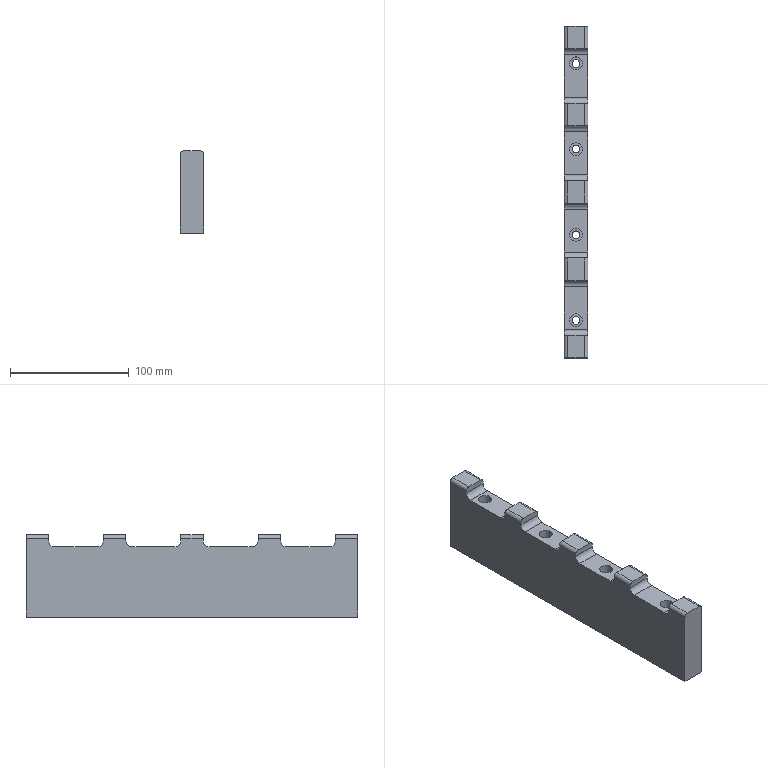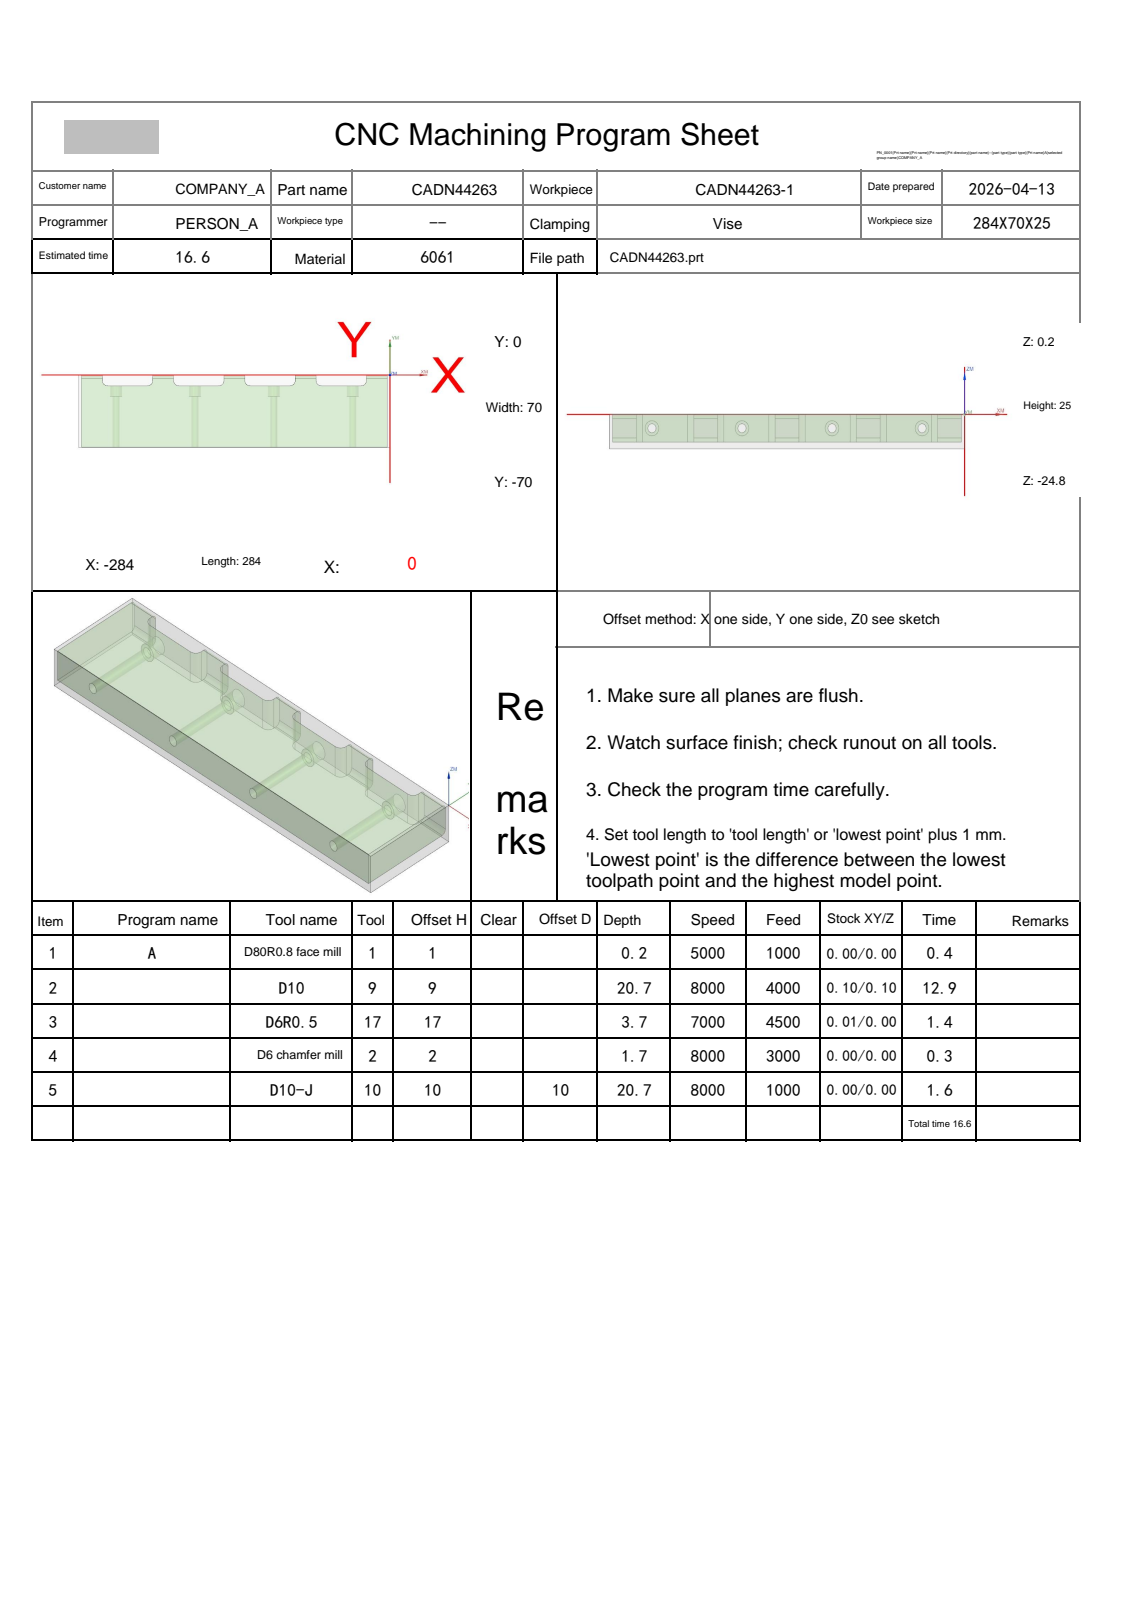NC program | NX | posted by the shop | part box 20 x 279 x 69 mm
Lines 32 to 993 of 9859:
N2 T09 M06
(D10  D=10. R=0. H=09 ce=0.10 di=0.10)
G00 G90 G54 X-229.134 Y12. M03 S8000
G43 H09 Z10.2
M08
Z.614
G01 Z-.586 F4000.
G02 X-228.084 Y8.312 I-5.95 J-3.688
X-228.918 Y5. I-7. J0.0
G03 X-229.323 Y4.183 I12.45 J-6.687
G02 X-230.23 Y3.6 I-.909 J.417
G01 X-248.795
G02 X-249.701 Y4.18 I.002 J1.
G03 X-250.111 Y5. I-12.905 J-5.942
G02 X-250.955 Y8.331 I6.156 J3.331
X-249.917 Y12. I7. J0.0
G01 Z.614
G00 Z3.
G01 X-164.121 F6000.
G00 Z.614
G01 Z-.586 F4000.
G02 X-163.073 Y8.315 I-5.952 J-3.685
X-163.908 Y5. I-7. J0.0
G03 X-164.314 Y4.183 I12.457 J-6.699
G02 X-165.221 Y3.6 I-.909 J.417
G01 X-183.777
G02 X-184.684 Y4.182 I.002 J1.
G03 X-185.091 Y5. I-12.87 J-5.892
G02 X-185.927 Y8.318 I6.164 J3.318
X-184.881 Y12. I7. J0.0
G01 Z.614
G00 Z3.
G01 X-99.102 F6000.
G00 Z.614
G01 Z-.586 F4000.
G02 X-98.06 Y8.324 I-5.957 J-3.676
X-98.9 Y5. I-7. J0.0
G03 X-99.308 Y4.181 I12.478 J-6.734
G02 X-100.214 Y3.6 I-.908 J.419
G01 X-118.771
G02 X-119.679 Y4.185 I.002 J1.
G03 X-120.081 Y5. I-12.821 J-5.821
G02 X-120.907 Y8.299 I6.174 J3.299
X-119.849 Y12. I7. J0.0
G01 Z.614
G00 Z3.
G01 X-34.092 F6000.
G00 Z.614
G01 Z-.586 F4000.
G02 X-33.051 Y8.328 I-5.96 J-3.672
X-33.893 Y5. I-7. J0.0
G03 X-34.303 Y4.181 I12.488 J-6.75
G02 X-35.209 Y3.6 I-.908 J.419
G01 X-53.77
G02 X-54.671 Y4.17 I.002 J1.
G03 X-55.573 Y4.739 I-.903 J-.431
X-55.932 Y4.673 I0.0 J-1.
G01 X-62.489 Y2.148
G03 X-63.13 Y1.214 I.359 J-.933
X-63.011 Y.741 I1. J0.0
G02 X-62.4 Y-1.687 I-4.521 J-2.429
G01 Y-1.72
Y-2.023
G03 X-62.225 Y-2.242 I.224 J0.0
G02 X-61.631 Y-2.785 I-.177 J-.79
G03 X-59.25 Y-4.523 I2.381 J.762
X-57.559 Y-3.865 I0.0 J2.5
G01 X-53.852 Y-.461
G03 X-53.043 Y1.381 I-1.691 J1.841
X-55.543 Y3.881 I-2.5 J0.0
X-57.234 Y3.222 I0.0 J-2.5
G01 X-60.941 Y-.182
G03 X-61.684 Y-1.452 I1.691 J-1.841
G02 X-61.993 Y-1.756 I-.394 J.093
G01 X-62.223 Y-1.805
G03 X-62.4 Y-2.023 I.047 J-.219
G01 Y-3.419
G02 X-62.379 Y-4.409 I-23.84 J-.991
X-62.4 Y-5.4 I-23.861 J0.0
G01 X-26.6
Y-2.028
G03 X-26.774 Y-1.81 I-.223 J0.0
G02 X-27.365 Y-1.269 I.177 J.787
G03 X-28.052 Y-.191 I-2.382 J-.759
G01 X-31.744 Y3.217
G03 X-33.439 Y3.88 I-1.696 J-1.837
X-35.939 Y1.38 I0.0 J-2.5
X-35.135 Y-.457 I2.5 J0.0
G01 X-31.443 Y-3.865
G03 X-29.747 Y-4.528 I1.696 J1.837
X-27.313 Y-2.597 I0.0 J2.5
G02 X-27.005 Y-2.294 I.393 J-.092
G01 X-26.776 Y-2.246
G03 X-26.6 Y-2.028 I-.046 J.218
G01 Y-1.844
X-26.601 Y-1.75
G02 X-21.5 Y3.445 I5.195 J0.0
G01 X-2.5
G02 X2.6 Y-1.713 I-.057 J-5.157
G01 Y-1.72
Y-69.443
Y-69.498
G02 X2.505 Y-70.479 I-5.101 J0.0
X-2.5 Y-74.6 I-5.005 J.979
G01 X-281.5
G02 X-286.505 Y-70.479 I0.0 J5.1
X-286.6 Y-69.498 I5.006 J.981
G01 Y-69.443
Y-1.72
Y-1.717
G02 X-281.5 Y3.445 I5.162 J0.0
G01 X-262.5
G02 X-257.399 Y-1.762 I-.107 J-5.207
G01 X-257.4 Y-1.869
Y-2.029
G03 X-257.226 Y-2.246 I.223 J0.0
G02 X-256.635 Y-2.787 I-.177 J-.786
G03 X-254.253 Y-4.529 I2.382 J.758
X-252.557 Y-3.865 I0.0 J2.5
G01 X-248.868 Y-.457
G03 X-248.064 Y1.379 I-1.696 J1.836
X-250.564 Y3.879 I-2.5 J0.0
X-252.261 Y3.216 I0.0 J-2.5
G01 X-255.95 Y-.192
G03 X-256.688 Y-1.46 I1.696 J-1.836
G02 X-256.995 Y-1.762 I-.392 J.092
G01 X-257.224 Y-1.811
G03 X-257.4 Y-2.029 I.046 J-.218
G01 Y-3.403
G02 X-257.378 Y-4.402 I-22.182 J-.998
X-257.4 Y-5.4 I-22.205 J0.0
G01 X-221.6
Y-2.023
G03 X-221.775 Y-1.805 I-.224 J0.0
G02 X-222.369 Y-1.262 I.177 J.79
G03 X-223.059 Y-.182 I-2.381 J-.762
G01 X-226.766 Y3.222
G03 X-228.457 Y3.881 I-1.691 J-1.841
X-230.957 Y1.381 I0.0 J-2.5
X-230.148 Y-.461 I2.5 J0.0
G01 X-226.441 Y-3.865
G03 X-224.75 Y-4.523 I1.691 J1.841
X-222.316 Y-2.594 I0.0 J2.5
G02 X-222.007 Y-2.291 I.394 J-.093
G01 X-221.777 Y-2.242
G03 X-221.6 Y-2.023 I-.047 J.219
G01 Y-1.72
Y-1.687
G02 X-216.5 Y3.445 I5.132 J0.0
G01 X-197.5
G02 X-192.4 Y-1.709 I-.054 J-5.154
G01 Y-1.763
Y-2.025
G03 X-192.225 Y-2.243 I.223 J0.0
G02 X-191.632 Y-2.785 I-.177 J-.789
G03 X-189.251 Y-4.525 I2.381 J.761
X-187.558 Y-3.865 I0.0 J2.5
G01 X-183.857 Y-.459
G03 X-183.049 Y1.38 I-1.693 J1.84
X-185.549 Y3.88 I-2.5 J0.0
X-187.242 Y3.22 I0.0 J-2.5
G01 X-190.943 Y-.185
G03 X-191.685 Y-1.455 I1.693 J-1.84
G02 X-191.994 Y-1.758 I-.394 J.092
G01 X-192.223 Y-1.807
G03 X-192.4 Y-2.025 I.047 J-.218
G01 Y-3.41
G02 X-192.382 Y-4.405 I-27.479 J-.995
X-192.4 Y-5.4 I-27.497 J0.0
G01 X-156.6
Y-5.388
G02 X-156.627 Y-4.37 I19.024 J1.018
X-156.6 Y-3.351 I19.052 J0.0
G01 Y-2.026
G03 X-156.773 Y-1.81 I-.222 J0.0
G02 X-157.362 Y-1.269 I.176 J.783
G03 X-158.051 Y-.187 I-2.383 J-.757
G01 X-161.752 Y3.222
G03 X-163.446 Y3.883 I-1.694 J-1.839
X-165.946 Y1.383 I0.0 J-2.5
X-165.14 Y-.456 I2.5 J0.0
G01 X-161.439 Y-3.865
G03 X-159.745 Y-4.526 I1.694 J1.839
X-157.31 Y-2.593 I0.0 J2.5
G02 X-157.003 Y-2.292 I.391 J-.091
G01 X-156.775 Y-2.243
G03 X-156.6 Y-2.026 I-.046 J.217
G01 Y-1.779
G02 X-156.454 Y-.505 I5.64 J0.0
X-151.5 Y3.445 I5.003 J-1.194
G01 X-132.5
G02 X-127.448 Y-1.094 I0.0 J-5.08
X-127.4 Y-2.002 I-8.464 J-.907
G01 Y-2.02
G03 X-127.23 Y-2.232 I.218 J0.0
G02 X-126.653 Y-2.766 I-.175 J-.769
G03 X-124.267 Y-4.52 I2.386 J.746
X-122.58 Y-3.865 I0.0 J2.5
G01 X-118.86 Y-.463
G03 X-118.047 Y1.382 I-1.687 J1.845
X-120.547 Y3.882 I-2.5 J0.0
X-122.234 Y3.227 I0.0 J-2.5
G01 X-125.954 Y-.175
G03 X-126.704 Y-1.462 I1.687 J-1.845
G02 X-127.005 Y-1.759 I-.384 J.088
G01 X-127.228 Y-1.807
G03 X-127.4 Y-2.02 I.046 J-.213
G01 Y-3.351
G02 X-127.372 Y-4.376 I-19.025 J-1.024
X-127.4 Y-5.4 I-19.052 J0.0
G01 X-91.6
Y-2.027
G03 X-91.774 Y-1.809 I-.223 J0.0
G02 X-92.366 Y-1.267 I.177 J.788
G03 X-93.054 Y-.188 I-2.382 J-.76
G01 X-96.749 Y3.218
G03 X-98.444 Y3.88 I-1.694 J-1.838
X-100.944 Y1.38 I0.0 J-2.5
X-100.138 Y-.458 I2.5 J0.0
G01 X-96.443 Y-3.865
G03 X-94.748 Y-4.527 I1.694 J1.838
X-92.314 Y-2.596 I0.0 J2.5
G02 X-92.005 Y-2.294 I.393 J-.092
G01 X-91.776 Y-2.245
G03 X-91.6 Y-2.027 I-.047 J.218
G01 Y-1.812
X-91.601 Y-1.734
G02 X-86.5 Y3.445 I5.179 J0.0
G01 X-67.5
G02 X-62.4 Y-1.687 I-.032 J-5.132
G01 Y-1.72
Y-3.419
G02 X-62.381 Y-4.157 I-23.84 J-.986
X-62.38 Y-4.405 I-23.859 J-.248
X-62.381 Y-4.657 I-23.861 J0.0
G03 X-55.381 Y2.343 I0.0 J7.
G01 Y12.
Z.614
G00 Z3.
G01 X-229.72 F6000.
G00 Z.029
G01 Z-1.171 F4000.
G02 X-228.495 Y8.044 I-5.775 J-3.956
X-229.191 Y5. I-7. J0.0
G03 X-229.54 Y4.218 I12.752 J-6.157
G02 X-230.462 Y3.6 I-.924 J.382
G01 X-248.523
G02 X-249.445 Y4.22 I.003 J1.
G03 X-249.791 Y5. I-13.068 J-5.329
G02 X-250.481 Y8.03 I6.31 J3.03
X-249.246 Y12. I7. J0.0
G01 Z.029
G00 Z2.414
G01 X-164.725 F6000.
G00 Z.029
G01 Z-1.171 F4000.
G02 X-163.499 Y8.042 I-5.774 J-3.958
X-164.194 Y5. I-7. J0.0
G03 X-164.543 Y4.218 I12.748 J-6.151
G02 X-165.464 Y3.6 I-.924 J.382
G01 X-183.523
G02 X-184.445 Y4.22 I.003 J1.
G03 X-184.791 Y5. I-13.068 J-5.329
G02 X-185.481 Y8.03 I6.31 J3.03
X-184.246 Y12. I7. J0.0
G01 Z.029
G00 Z2.414
G01 X-99.754 F6000.
G00 Z.029
G01 Z-1.171 F4000.
G02 X-98.519 Y8.03 I-5.765 J-3.97
X-99.209 Y5. I-7. J0.0
G03 X-99.555 Y4.22 I12.722 J-6.109
G02 X-100.477 Y3.6 I-.925 J.38
G01 X-118.523
G02 X-119.445 Y4.22 I.003 J1.
G03 X-119.791 Y5. I-13.068 J-5.329
G02 X-120.481 Y8.03 I6.31 J3.03
X-119.246 Y12. I7. J0.0
G01 Z.029
G00 Z2.414
G01 X-34.754 F6000.
G00 Z.029
G01 Z-1.171 F4000.
G02 X-33.519 Y8.03 I-5.765 J-3.97
X-34.209 Y5. I-7. J0.0
G03 X-34.555 Y4.22 I12.722 J-6.109
G02 X-35.477 Y3.6 I-.925 J.38
G01 X-53.538
G02 X-54.444 Y4.181 I.003 J1.
G03 X-55.352 Y4.762 I-.908 J-.419
X-55.67 Y4.71 I0.0 J-1.
G01 X-62.332 Y2.469
G03 X-63.013 Y1.522 I.319 J-.948
X-62.913 Y1.087 I1. J0.0
G02 X-62.4 Y-1.121 I-4.648 J-2.244
G01 Y-1.989
G03 X-62.218 Y-2.215 I.232 J0.0
G02 X-61.601 Y-2.772 I-.18 J-.82
G03 X-59.227 Y-4.489 I2.374 J.783
X-57.572 Y-3.863 I0.0 J2.5
G01 X-53.717 Y-.458
G03 X-52.873 Y1.416 I-1.655 J1.874
X-55.373 Y3.916 I-2.5 J0.0
X-57.028 Y3.29 I0.0 J-2.5
G01 X-60.882 Y-.115
G03 X-61.656 Y-1.4 I1.655 J-1.874
G02 X-61.977 Y-1.711 I-.408 J.099
G01 X-62.216 Y-1.762
G03 X-62.4 Y-1.989 I.048 J-.227
G01 Y-3.419
G02 X-62.379 Y-4.409 I-23.84 J-.991
X-62.4 Y-5.4 I-23.861 J0.0
G01 X-26.6
Y-1.985
G03 X-26.782 Y-1.759 I-.232 J0.0
G02 X-27.399 Y-1.202 I.18 J.82
G03 X-28.122 Y-.108 I-2.374 J-.783
G01 X-31.989 Y3.294
G03 X-33.64 Y3.917 I-1.651 J-1.877
X-36.14 Y1.417 I0.0 J-2.5
X-35.292 Y-.46 I2.5 J0.0
G01 X-31.425 Y-3.862
G03 X-29.773 Y-4.485 I1.651 J1.877
X-27.344 Y-2.574 I0.0 J2.5
G02 X-27.023 Y-2.263 I.408 J-.099
G01 X-26.784 Y-2.212
G03 X-26.6 Y-1.985 I-.048 J.227
G01 Y-1.121
Y-1.109
G02 X-21.5 Y4.003 I5.112 J0.0
G01 X-2.5
G02 X2.6 Y-1.109 I-.012 J-5.112
G01 Y-1.121
Y-69.443
Y-69.498
G02 X2.505 Y-70.479 I-5.101 J0.0
X-2.5 Y-74.6 I-5.005 J.979
G01 X-281.5
G02 X-286.505 Y-70.479 I0.0 J5.1
X-286.6 Y-69.498 I5.006 J.981
G01 Y-69.443
Y-1.121
Y-1.109
G02 X-281.5 Y4.003 I5.112 J0.0
G01 X-262.5
G02 X-257.4 Y-1.109 I-.012 J-5.112
G01 Y-1.121
Y-1.655
X-257.398 Y-1.749
G03 X-257.18 Y-2.092 I.386 J.005
G01 X-256.944 Y-2.205
G02 X-256.66 Y-2.559 I-.23 J-.475
G03 X-254.227 Y-4.485 I2.433 J.574
X-252.575 Y-3.862 I0.0 J2.5
G01 X-248.708 Y-.46
G03 X-247.86 Y1.417 I-1.651 J1.877
X-250.36 Y3.917 I-2.5 J0.0
X-252.011 Y3.294 I0.0 J-2.5
G01 X-255.878 Y-.108
G03 X-256.656 Y-1.396 I1.651 J-1.877
G02 X-256.977 Y-1.708 I-.408 J.099
G01 X-257.216 Y-1.759
G03 X-257.4 Y-1.985 I.048 J-.227
G01 Y-3.403
G02 X-257.378 Y-4.402 I-22.182 J-.998
X-257.4 Y-5.4 I-22.205 J0.0
G01 X-221.6
Y-1.989
G03 X-221.782 Y-1.763 I-.232 J0.0
G02 X-222.399 Y-1.206 I.18 J.82
G03 X-223.118 Y-.115 I-2.374 J-.783
G01 X-226.972 Y3.29
G03 X-228.627 Y3.916 I-1.655 J-1.874
X-231.127 Y1.416 I0.0 J-2.5
X-230.283 Y-.458 I2.5 J0.0
G01 X-226.428 Y-3.863
G03 X-224.773 Y-4.489 I1.655 J1.874
X-222.344 Y-2.578 I0.0 J2.5
G02 X-222.023 Y-2.267 I.408 J-.099
G01 X-221.784 Y-2.216
G03 X-221.6 Y-1.989 I-.048 J.227
G01 Y-1.121
G02 X-216.5 Y4.003 I5.161 J-.036
G01 X-197.5
G02 X-192.4 Y-1.109 I-.012 J-5.112
G01 Y-1.121
Y-1.985
G03 X-192.218 Y-2.212 I.232 J0.0
G02 X-191.601 Y-2.768 I-.18 J-.82
G03 X-189.227 Y-4.485 I2.374 J.783
X-187.575 Y-3.862 I0.0 J2.5
G01 X-183.708 Y-.46
G03 X-182.86 Y1.417 I-1.651 J1.877
X-185.36 Y3.917 I-2.5 J0.0
X-187.011 Y3.294 I0.0 J-2.5
G01 X-190.878 Y-.108
G03 X-191.656 Y-1.396 I1.651 J-1.877
G02 X-191.977 Y-1.708 I-.408 J.099
G01 X-192.216 Y-1.759
G03 X-192.4 Y-1.985 I.048 J-.227
G01 Y-3.41
G02 X-192.382 Y-4.405 I-27.479 J-.995
X-192.4 Y-5.4 I-27.497 J0.0
G01 X-156.6
Y-5.388
G02 X-156.627 Y-4.37 I19.024 J1.018
X-156.6 Y-3.351 I19.052 J0.0
G01 Y-1.989
G03 X-156.782 Y-1.762 I-.232 J0.0
G02 X-157.4 Y-1.205 I.18 J.82
G03 X-158.119 Y-.114 I-2.374 J-.783
G01 X-161.975 Y3.29
G03 X-163.629 Y3.916 I-1.655 J-1.874
X-166.129 Y1.416 I0.0 J-2.5
X-165.284 Y-.458 I2.5 J0.0
G01 X-161.428 Y-3.863
G03 X-159.774 Y-4.489 I1.655 J1.874
X-157.344 Y-2.578 I0.0 J2.5
G02 X-157.024 Y-2.266 I.408 J-.099
G01 X-156.784 Y-2.215
G03 X-156.6 Y-1.989 I-.048 J.227
G01 Y-1.62
Y-1.121
G02 X-151.5 Y4.003 I5.155 J-.03
G01 X-132.5
G02 X-127.4 Y-1.109 I-.012 J-5.112
G01 Y-1.121
Y-1.985
G03 X-127.218 Y-2.212 I.232 J0.0
G02 X-126.601 Y-2.768 I-.18 J-.82
G03 X-124.227 Y-4.485 I2.374 J.783
X-122.575 Y-3.862 I0.0 J2.5
G01 X-118.708 Y-.46
G03 X-117.86 Y1.417 I-1.651 J1.877
X-120.36 Y3.917 I-2.5 J0.0
X-122.011 Y3.294 I0.0 J-2.5
G01 X-125.878 Y-.108
G03 X-126.656 Y-1.396 I1.651 J-1.877
G02 X-126.977 Y-1.708 I-.408 J.099
G01 X-127.216 Y-1.759
G03 X-127.4 Y-1.985 I.048 J-.227
G01 Y-3.351
G02 X-127.372 Y-4.376 I-19.025 J-1.024
X-127.4 Y-5.4 I-19.052 J0.0
G01 X-91.6
Y-1.985
G03 X-91.782 Y-1.759 I-.232 J0.0
G02 X-92.399 Y-1.202 I.18 J.82
G03 X-93.122 Y-.108 I-2.374 J-.783
G01 X-96.989 Y3.294
G03 X-98.64 Y3.917 I-1.651 J-1.877
X-101.14 Y1.417 I0.0 J-2.5
X-100.292 Y-.46 I2.5 J0.0
G01 X-96.425 Y-3.862
G03 X-94.773 Y-4.485 I1.651 J1.877
X-92.344 Y-2.574 I0.0 J2.5
G02 X-92.023 Y-2.263 I.408 J-.099
G01 X-91.784 Y-2.212
G03 X-91.6 Y-1.985 I-.048 J.227
G01 Y-1.121
Y-1.109
G02 X-86.5 Y4.003 I5.112 J0.0
G01 X-67.5
G02 X-62.4 Y-1.121 I-.061 J-5.161
G01 Y-3.419
G02 X-62.386 Y-3.836 I-23.84 J-.986
X-62.38 Y-4.336 I-23.854 J-.57
G03 X-55.38 Y2.664 I0.0 J7.
G01 Y12.
Z.029
G00 Z2.414
G01 X-230.111 F6000.
G00 Z-.557
G01 Z-1.757 F4000.
G02 X-228.757 Y7.861 I-5.645 J-4.139
X-229.368 Y5. I-7. J0.0
G03 X-229.681 Y4.242 I12.873 J-5.765
G02 X-230.612 Y3.6 I-.934 J.358
G01 X-248.388
G02 X-249.319 Y4.242 I.003 J1.
G03 X-249.632 Y5. I-13.186 J-5.007
G02 X-250.243 Y7.861 I6.389 J2.861
X-248.889 Y12. I7. J0.0
G01 Z-.557
G00 Z1.829
G01 X-165.111 F6000.
G00 Z-.557
G01 Z-1.757 F4000.
G02 X-163.757 Y7.861 I-5.645 J-4.139
X-164.368 Y5. I-7. J0.0
G03 X-164.681 Y4.242 I12.873 J-5.765
G02 X-165.612 Y3.6 I-.934 J.358
G01 X-183.388
G02 X-184.319 Y4.242 I.003 J1.
G03 X-184.632 Y5. I-13.186 J-5.007
G02 X-185.243 Y7.861 I6.389 J2.861
X-183.889 Y12. I7. J0.0
G01 Z-.557
G00 Z1.829
G01 X-100.1 F6000.
G00 Z-.557
G01 Z-1.757 F4000.
G02 X-98.749 Y7.866 I-5.649 J-4.134
X-99.362 Y5. I-7. J0.0
G03 X-99.676 Y4.242 I12.884 J-5.782
G02 X-100.607 Y3.6 I-.934 J.358
G01 X-118.388
G02 X-119.319 Y4.242 I.003 J1.
G03 X-119.632 Y5. I-13.186 J-5.007
G02 X-120.243 Y7.861 I6.389 J2.861
X-118.889 Y12. I7. J0.0
G01 Z-.557
G00 Z1.829
G01 X-35.111 F6000.
G00 Z-.557
G01 Z-1.757 F4000.
G02 X-33.757 Y7.861 I-5.645 J-4.139
X-34.368 Y5. I-7. J0.0
G03 X-34.681 Y4.242 I12.873 J-5.765
G02 X-35.612 Y3.6 I-.934 J.358
G01 X-53.388
G02 X-54.297 Y4.19 I.003 J1.
G03 X-55.209 Y4.779 I-.912 J-.411
X-55.5 Y4.736 I0.0 J-1.
G01 X-62.225 Y2.687
G03 X-62.933 Y1.73 I.291 J-.957
X-62.846 Y1.321 I1. J0.0
G02 X-62.4 Y-.765 I-4.659 J-2.087
G01 Y-.77
Y-1.962
G03 X-62.218 Y-2.188 I.231 J0.0
G02 X-61.603 Y-2.744 I-.18 J-.818
G03 X-59.228 Y-4.462 I2.375 J.782
X-57.601 Y-3.86 I0.0 J2.5
G01 X-53.635 Y-.459
G03 X-52.763 Y1.439 I-1.628 J1.898
X-55.263 Y3.939 I-2.5 J0.0
X-56.89 Y3.336 I0.0 J-2.5
G01 X-60.856 Y-.065
G03 X-61.658 Y-1.375 I1.628 J-1.898
G02 X-61.978 Y-1.685 I-.407 J.099
G01 X-62.217 Y-1.736
G03 X-62.4 Y-1.962 I.048 J-.226
G01 Y-3.419
G02 X-62.379 Y-4.409 I-23.84 J-.991
X-62.4 Y-5.4 I-23.861 J0.0
G01 X-26.6
Y-1.962
G03 X-26.782 Y-1.737 I-.231 J0.0
G02 X-27.397 Y-1.181 I.18 J.818
G03 X-28.144 Y-.065 I-2.375 J-.782
G01 X-32.11 Y3.336
G03 X-33.737 Y3.939 I-1.628 J-1.898
X-36.237 Y1.439 I0.0 J-2.5
X-35.365 Y-.459 I2.5 J0.0
G01 X-31.399 Y-3.86
G03 X-29.772 Y-4.462 I1.628 J1.898
X-27.342 Y-2.55 I0.0 J2.5
G02 X-27.022 Y-2.239 I.407 J-.099
G01 X-26.783 Y-2.189
G03 X-26.6 Y-1.962 I-.048 J.226
G01 Y-.77
Y-.765
G02 X-21.5 Y4.34 I5.105 J0.0
G01 X-2.5
G02 X2.6 Y-.765 I-.005 J-5.105
G01 Y-.77
Y-69.443
Y-69.498
G02 X2.505 Y-70.478 I-5.101 J0.0
X-2.5 Y-74.6 I-5.005 J.978
G01 X-281.5
G02 X-286.505 Y-70.479 I0.0 J5.1
X-286.6 Y-69.498 I5.006 J.981
G01 Y-69.443
Y-.77
Y-.765
G02 X-281.5 Y4.34 I5.105 J0.0
G01 X-262.5
G02 X-257.4 Y-.765 I-.005 J-5.105
G01 Y-.77
Y-1.962
G03 X-257.218 Y-2.188 I.231 J0.0
G02 X-256.603 Y-2.744 I-.18 J-.818
G03 X-254.228 Y-4.462 I2.375 J.782
X-252.601 Y-3.86 I0.0 J2.5
G01 X-248.635 Y-.459
G03 X-247.763 Y1.439 I-1.628 J1.898
X-250.263 Y3.939 I-2.5 J0.0
X-251.89 Y3.336 I0.0 J-2.5
G01 X-255.856 Y-.065
G03 X-256.658 Y-1.375 I1.628 J-1.898
G02 X-256.978 Y-1.685 I-.407 J.099
G01 X-257.217 Y-1.736
G03 X-257.4 Y-1.962 I.048 J-.226
G01 Y-3.403
G02 X-257.378 Y-4.402 I-22.182 J-.998
X-257.4 Y-5.4 I-22.205 J0.0
G01 X-221.6
Y-1.962
G03 X-221.782 Y-1.737 I-.231 J0.0
G02 X-222.397 Y-1.181 I.18 J.818
G03 X-223.144 Y-.065 I-2.375 J-.782
G01 X-227.11 Y3.336
G03 X-228.737 Y3.939 I-1.628 J-1.898
X-231.237 Y1.439 I0.0 J-2.5
X-230.365 Y-.459 I2.5 J0.0
G01 X-226.399 Y-3.86
G03 X-224.772 Y-4.462 I1.628 J1.898
X-222.342 Y-2.55 I0.0 J2.5
G02 X-222.022 Y-2.239 I.407 J-.099
G01 X-221.783 Y-2.189
G03 X-221.6 Y-1.962 I-.048 J.226
G01 Y-.77
Y-.765
G02 X-216.5 Y4.34 I5.105 J0.0
G01 X-197.5
G02 X-192.4 Y-.765 I-.005 J-5.105
G01 Y-.77
Y-1.962
G03 X-192.218 Y-2.188 I.231 J0.0
G02 X-191.603 Y-2.744 I-.18 J-.818
G03 X-189.228 Y-4.462 I2.375 J.782
X-187.601 Y-3.86 I0.0 J2.5
G01 X-183.635 Y-.459
G03 X-182.763 Y1.439 I-1.628 J1.898
X-185.263 Y3.939 I-2.5 J0.0
X-186.89 Y3.336 I0.0 J-2.5
G01 X-190.856 Y-.065
G03 X-191.658 Y-1.375 I1.628 J-1.898
G02 X-191.978 Y-1.685 I-.407 J.099
G01 X-192.217 Y-1.736
G03 X-192.4 Y-1.962 I.048 J-.226
G01 Y-3.41
G02 X-192.382 Y-4.405 I-27.479 J-.995
X-192.4 Y-5.4 I-27.497 J0.0
G01 X-156.6
Y-5.388
G02 X-156.627 Y-4.37 I19.024 J1.018
X-156.6 Y-3.351 I19.052 J0.0
G01 Y-1.962
G03 X-156.782 Y-1.737 I-.231 J0.0
G02 X-157.397 Y-1.181 I.18 J.818
G03 X-158.144 Y-.065 I-2.375 J-.782
G01 X-162.11 Y3.336
G03 X-163.737 Y3.939 I-1.628 J-1.898
X-166.237 Y1.439 I0.0 J-2.5
X-165.365 Y-.459 I2.5 J0.0
G01 X-161.399 Y-3.86
G03 X-159.772 Y-4.462 I1.628 J1.898
X-157.342 Y-2.55 I0.0 J2.5
G02 X-157.022 Y-2.239 I.407 J-.099
G01 X-156.783 Y-2.189
G03 X-156.6 Y-1.962 I-.048 J.226
G01 Y-1.62
Y-.77
Y-.765
G02 X-151.5 Y4.34 I5.105 J0.0
G01 X-132.5
G02 X-127.4 Y-.765 I-.005 J-5.105
G01 Y-.77
Y-1.962
G03 X-127.218 Y-2.188 I.231 J0.0
G02 X-126.603 Y-2.744 I-.18 J-.818
G03 X-124.228 Y-4.462 I2.375 J.782
X-122.601 Y-3.86 I0.0 J2.5
G01 X-118.635 Y-.459
G03 X-117.763 Y1.439 I-1.628 J1.898
X-120.263 Y3.939 I-2.5 J0.0
X-121.89 Y3.336 I0.0 J-2.5
G01 X-125.856 Y-.065
G03 X-126.658 Y-1.375 I1.628 J-1.898
G02 X-126.978 Y-1.685 I-.407 J.099
G01 X-127.217 Y-1.736
G03 X-127.4 Y-1.962 I.048 J-.226
G01 Y-3.351
G02 X-127.372 Y-4.376 I-19.025 J-1.024
X-127.4 Y-5.4 I-19.052 J0.0
G01 X-91.6
Y-1.964
G03 X-91.782 Y-1.738 I-.231 J0.0
G02 X-92.398 Y-1.182 I.18 J.818
G03 X-93.143 Y-.067 I-2.375 J-.782
G01 X-97.104 Y3.335
G03 X-98.733 Y3.938 I-1.629 J-1.896
X-101.233 Y1.438 I0.0 J-2.5
X-100.362 Y-.458 I2.5 J0.0
G01 X-96.401 Y-3.86
G03 X-94.772 Y-4.464 I1.629 J1.896
X-92.342 Y-2.552 I0.0 J2.5
G02 X-92.023 Y-2.241 I.407 J-.099
G01 X-91.783 Y-2.19
G03 X-91.6 Y-1.964 I-.048 J.226
G01 Y-.77
G02 X-86.5 Y4.34 I5.122 J-.012
G01 X-67.5
G02 X-62.4 Y-.765 I-.005 J-5.105
G01 Y-.77
Y-3.419
X-62.393 Y-3.615
G02 X-62.381 Y-4.115 I-23.848 J-.79
G03 X-55.381 Y2.885 I0.0 J7.
G01 Y12.
Z-.557
G00 Z1.829
G01 X-230.29 F6000.
G00 Z-1.143
G01 Z-2.343 F4000.
G02 X-228.871 Y7.774 I-5.58 J-4.226
X-229.444 Y5. I-7. J0.0
G03 X-229.741 Y4.253 I12.971 J-5.598
G02 X-230.675 Y3.6 I-.938 J.347
G01 X-248.324
G02 X-249.258 Y4.253 I.004 J1.
G03 X-249.556 Y5. I-13.267 J-4.849
G02 X-250.128 Y7.773 I6.427 J2.773
X-248.708 Y12. I7. J0.0
G01 Z-1.143
G00 Z1.243
G01 X-165.309 F6000.
G00 Z-1.143
G01 Z-2.343 F4000.
G02 X-163.883 Y7.766 I-5.574 J-4.234
X-164.453 Y5. I-7. J0.0
G03 X-164.749 Y4.254 I12.954 J-5.571
G02 X-165.683 Y3.6 I-.938 J.346
G01 X-183.317
G02 X-184.251 Y4.254 I.004 J1.
G03 X-184.547 Y5. I-13.25 J-4.826
G02 X-185.117 Y7.766 I6.43 J2.766
X-183.691 Y12. I7. J0.0
G01 Z-1.143
G00 Z1.243
G01 X-100.309 F6000.
G00 Z-1.143
G01 Z-2.343 F4000.
G02 X-98.883 Y7.766 I-5.574 J-4.234
X-99.453 Y5. I-7. J0.0
G03 X-99.749 Y4.254 I12.954 J-5.571
G02 X-100.683 Y3.6 I-.938 J.346
G01 X-118.317
G02 X-119.251 Y4.254 I.004 J1.
G03 X-119.547 Y5. I-13.25 J-4.826
G02 X-120.117 Y7.766 I6.43 J2.766
X-118.691 Y12. I7. J0.0
G01 Z-1.143
G00 Z1.243
G01 X-35.29 F6000.
G00 Z-1.143
G01 Z-2.343 F4000.
G02 X-33.871 Y7.774 I-5.58 J-4.226
X-34.444 Y5. I-7. J0.0
G03 X-34.741 Y4.253 I12.971 J-5.598
G02 X-35.675 Y3.6 I-.938 J.347
G01 X-53.325
G02 X-54.235 Y4.194 I.004 J1.
G03 X-55.148 Y4.787 I-.914 J-.407
X-55.426 Y4.748 I0.0 J-1.
G01 X-62.18 Y2.79
G03 X-62.902 Y1.83 I.278 J-.96
X-62.82 Y1.434 I1. J0.0
G02 X-62.4 Y-.572 I-4.708 J-2.032
G01 Y-1.952
G03 X-62.22 Y-2.176 I.23 J0.0
G02 X-61.609 Y-2.729 I-.179 J-.812
G03 X-59.233 Y-4.452 I2.376 J.777
X-57.617 Y-3.859 I0.0 J2.5
G01 X-53.602 Y-.457
G03 X-52.718 Y1.45 I-1.616 J1.907
X-55.218 Y3.95 I-2.5 J0.0
X-56.835 Y3.358 I0.0 J-2.5
G01 X-60.849 Y-.044
G03 X-61.687 Y-1.476 I1.616 J-1.907
G02 X-61.825 Y-1.729 I-.471 J.091
G01 X-62.156 Y-2.05
G03 X-62.4 Y-2.624 I.556 J-.575
G01 Y-3.419
G02 X-62.379 Y-4.409 I-23.84 J-.991
X-62.4 Y-5.4 I-23.861 J0.0
G01 X-26.6
Y-1.952
G03 X-26.78 Y-1.727 I-.23 J0.0
G02 X-27.391 Y-1.174 I.179 J.812
G03 X-28.151 Y-.044 I-2.376 J-.777
G01 X-32.166 Y3.358
G03 X-33.782 Y3.95 I-1.616 J-1.907
X-36.282 Y1.45 I0.0 J-2.5
X-35.398 Y-.457 I2.5 J0.0
G01 X-31.383 Y-3.859
G03 X-29.767 Y-4.452 I1.616 J1.907
X-27.336 Y-2.536 I0.0 J2.5
G02 X-27.019 Y-2.227 I.404 J-.097
G01 X-26.782 Y-2.176
G03 X-26.6 Y-1.952 I-.048 J.225
G01 Y-.573
G02 X-21.5 Y4.53 I5.128 J-.025
G01 X-2.5
G02 X2.6 Y-.572 I-.03 J-5.13
G01 Y-69.443
Y-69.498
G02 X2.505 Y-70.478 I-5.101 J0.0
X-2.5 Y-74.6 I-5.005 J.978
G01 X-281.5
G02 X-286.505 Y-70.479 I0.0 J5.1
X-286.6 Y-69.498 I5.006 J.981
G01 Y-69.443
Y-.573
Y-.571
G02 X-281.5 Y4.53 I5.101 J0.0
G01 X-262.5
G02 X-257.4 Y-.572 I-.025 J-5.125
G01 Y-1.951
G03 X-257.22 Y-2.176 I.23 J0.0
G02 X-256.609 Y-2.729 I-.179 J-.812
G03 X-254.233 Y-4.451 I2.376 J.777
X-252.617 Y-3.859 I0.0 J2.5
G01 X-248.602 Y-.457
G03 X-247.718 Y1.451 I-1.616 J1.907
X-250.218 Y3.951 I-2.5 J0.0
X-251.834 Y3.358 I0.0 J-2.5
G01 X-255.849 Y-.044
G03 X-256.664 Y-1.367 I1.616 J-1.907
G02 X-256.981 Y-1.676 I-.404 J.097
G01 X-257.218 Y-1.727
G03 X-257.4 Y-1.951 I.048 J-.225
G01 Y-3.403
G02 X-257.378 Y-4.402 I-22.182 J-.998
X-257.4 Y-5.4 I-22.205 J0.0
G01 X-221.6
Y-1.952
G03 X-221.78 Y-1.727 I-.23 J0.0
G02 X-222.391 Y-1.174 I.179 J.812
G03 X-223.151 Y-.044 I-2.376 J-.777
G01 X-227.165 Y3.358
G03 X-228.782 Y3.95 I-1.616 J-1.907
X-231.282 Y1.45 I0.0 J-2.5
X-230.398 Y-.457 I2.5 J0.0
G01 X-226.383 Y-3.859
G03 X-224.767 Y-4.452 I1.616 J1.907
X-222.336 Y-2.536 I0.0 J2.5
G02 X-222.019 Y-2.227 I.404 J-.097
G01 X-221.782 Y-2.176
G03 X-221.6 Y-1.952 I-.048 J.225
G01 Y-.573
G02 X-216.5 Y4.53 I5.128 J-.026
G01 X-197.5
G02 X-192.4 Y-.571 I-.001 J-5.101
G01 Y-1.95
G03 X-192.22 Y-2.173 I.229 J0.0
G02 X-191.611 Y-2.726 I-.179 J-.81
G03 X-189.234 Y-4.45 I2.377 J.776
X-187.62 Y-3.859 I0.0 J2.5
G01 X-183.598 Y-.458
G03 X-182.712 Y1.451 I-1.614 J1.909
X-185.212 Y3.951 I-2.5 J0.0
X-186.826 Y3.36 I0.0 J-2.5
G01 X-190.848 Y-.04
G03 X-191.665 Y-1.366 I1.614 J-1.909
G02 X-191.982 Y-1.675 I-.403 J.097
G01 X-192.219 Y-1.725
G03 X-192.4 Y-1.95 I.048 J-.224
G01 Y-3.41
G02 X-192.382 Y-4.405 I-27.479 J-.995
X-192.4 Y-5.4 I-27.497 J0.0
G01 X-156.6
Y-5.388
G02 X-156.627 Y-4.37 I19.024 J1.018
X-156.6 Y-3.351 I19.052 J0.0
G01 Y-1.95
G03 X-156.78 Y-1.726 I-.229 J0.0
G02 X-157.389 Y-1.173 I.179 J.81
G03 X-158.152 Y-.04 I-2.376 J-.776
G01 X-162.174 Y3.36
G03 X-163.788 Y3.951 I-1.614 J-1.909
X-166.288 Y1.451 I0.0 J-2.5
X-165.402 Y-.458 I2.5 J0.0
G01 X-161.38 Y-3.859
G03 X-159.766 Y-4.45 I1.614 J1.909
X-157.335 Y-2.533 I0.0 J2.5
G02 X-157.018 Y-2.224 I.403 J-.097
G01 X-156.781 Y-2.174
G03 X-156.6 Y-1.95 I-.048 J.224
G01 Y-1.62
Y-.573
Y-.571
G02 X-151.5 Y4.53 I5.101 J0.0
G01 X-132.5
G02 X-127.4 Y-.571 I-.001 J-5.101
G01 Y-1.95
G03 X-127.22 Y-2.173 I.229 J0.0
G02 X-126.611 Y-2.726 I-.179 J-.81
G03 X-124.234 Y-4.45 I2.376 J.776
X-122.62 Y-3.859 I0.0 J2.5
G01 X-118.598 Y-.458
G03 X-117.712 Y1.451 I-1.614 J1.909
X-120.212 Y3.951 I-2.5 J0.0
X-121.826 Y3.36 I0.0 J-2.5
G01 X-125.848 Y-.04
G03 X-126.665 Y-1.366 I1.614 J-1.909
G02 X-126.982 Y-1.675 I-.403 J.097
G01 X-127.219 Y-1.725
G03 X-127.4 Y-1.95 I.048 J-.224
G01 Y-3.351
G02 X-127.372 Y-4.376 I-19.025 J-1.024
X-127.4 Y-5.4 I-19.052 J0.0
G01 X-91.6
Y-1.95
G03 X-91.78 Y-1.726 I-.229 J0.0
G02 X-92.389 Y-1.173 I.179 J.81
G03 X-93.152 Y-.04 I-2.376 J-.776
G01 X-97.174 Y3.36
G03 X-98.788 Y3.951 I-1.614 J-1.909
X-101.288 Y1.451 I0.0 J-2.5
X-100.402 Y-.458 I2.5 J0.0
G01 X-96.38 Y-3.859
G03 X-94.766 Y-4.45 I1.614 J1.909
X-92.335 Y-2.533 I0.0 J2.5
G02 X-92.018 Y-2.224 I.403 J-.097
G01 X-91.781 Y-2.174
G03 X-91.6 Y-1.95 I-.048 J.224
G01 Y-.573
Y-.571
G02 X-86.5 Y4.53 I5.101 J0.0
G01 X-67.5
G02 X-62.4 Y-.572 I-.028 J-5.128
G01 Y-1.952
X-62.396 Y-3.509
G02 X-62.383 Y-4.009 I-23.844 J-.896
G03 X-55.383 Y2.991 I0.0 J7.
G01 Y12.
Z-1.143
G00 Z1.243
G01 X-230.381 F6000.
G00 Z-1.729
G01 Z-2.929 F4000.
G02 X-228.928 Y7.731 I-5.547 J-4.269
X-229.483 Y5. I-7. J0.0
G03 X-229.772 Y4.259 I12.982 J-5.5
G02 X-230.709 Y3.6 I-.94 J.341
G01 X-248.291
G02 X-249.228 Y4.259 I.004 J1.
G03 X-249.517 Y5. I-13.273 J-4.76
G02 X-250.072 Y7.731 I6.445 J2.731
X-248.62 Y12. I7. J0.0
G01 Z-1.729
G00 Z.657
G01 X-165.381 F6000.
G00 Z-1.729
G01 Z-2.929 F4000.
G02 X-163.928 Y7.731 I-5.547 J-4.269
X-164.483 Y5. I-7. J0.0
G03 X-164.773 Y4.259 I12.982 J-5.5
G02 X-165.709 Y3.6 I-.94 J.341
G01 X-183.291
G02 X-184.228 Y4.259 I.004 J1.
G03 X-184.517 Y5. I-13.273 J-4.76
G02 X-185.072 Y7.731 I6.445 J2.731
X-183.62 Y12. I7. J0.0
G01 Z-1.729
G00 Z.657
G01 X-100.38 F6000.